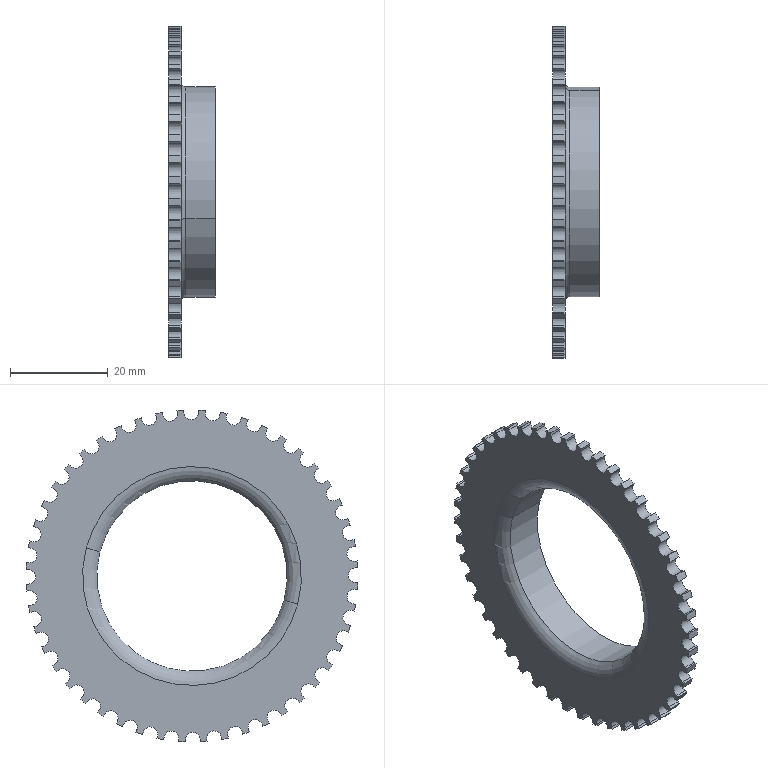Part | NX | features BREP 1 | 1 solid | 226 faces | box 9.5 x 67.946 x 67.946 mm | volume 7137 mm3 | cylinder 123 | plane 99 | torus 4 | commonest cylinder face diameters 3 x71 68 x48 39 x2 43 x2